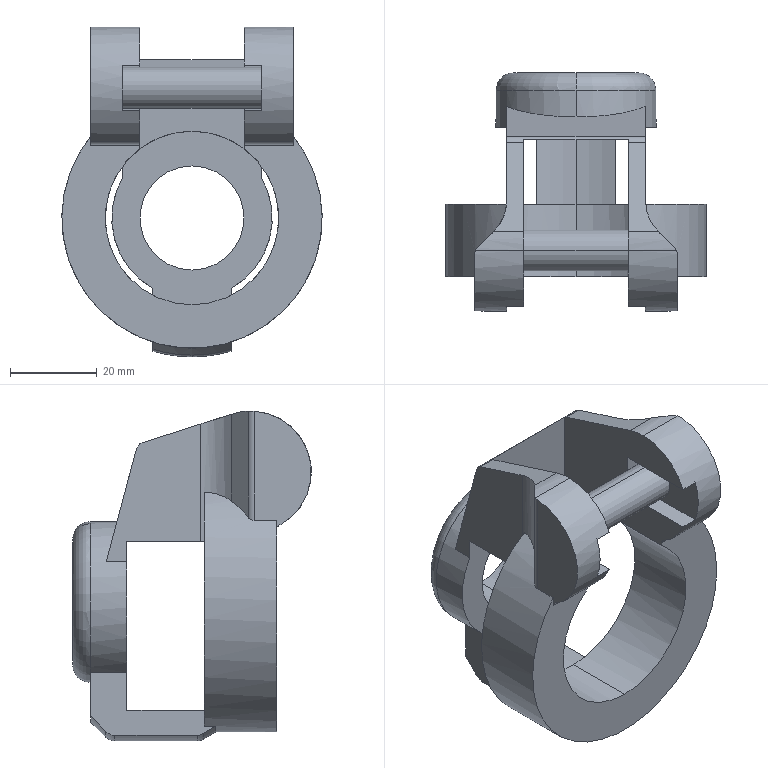Part | NX | features BREP 1 | 1 solid | 62 faces | box 60 x 55 x 76 mm | volume 47203 mm3 | plane 29 | cylinder 24 | torus 6 | cone 3 | commonest cylinder face diameters 28 x4 4 x3 2 x2 9.5 x2 20 x2 24 x2